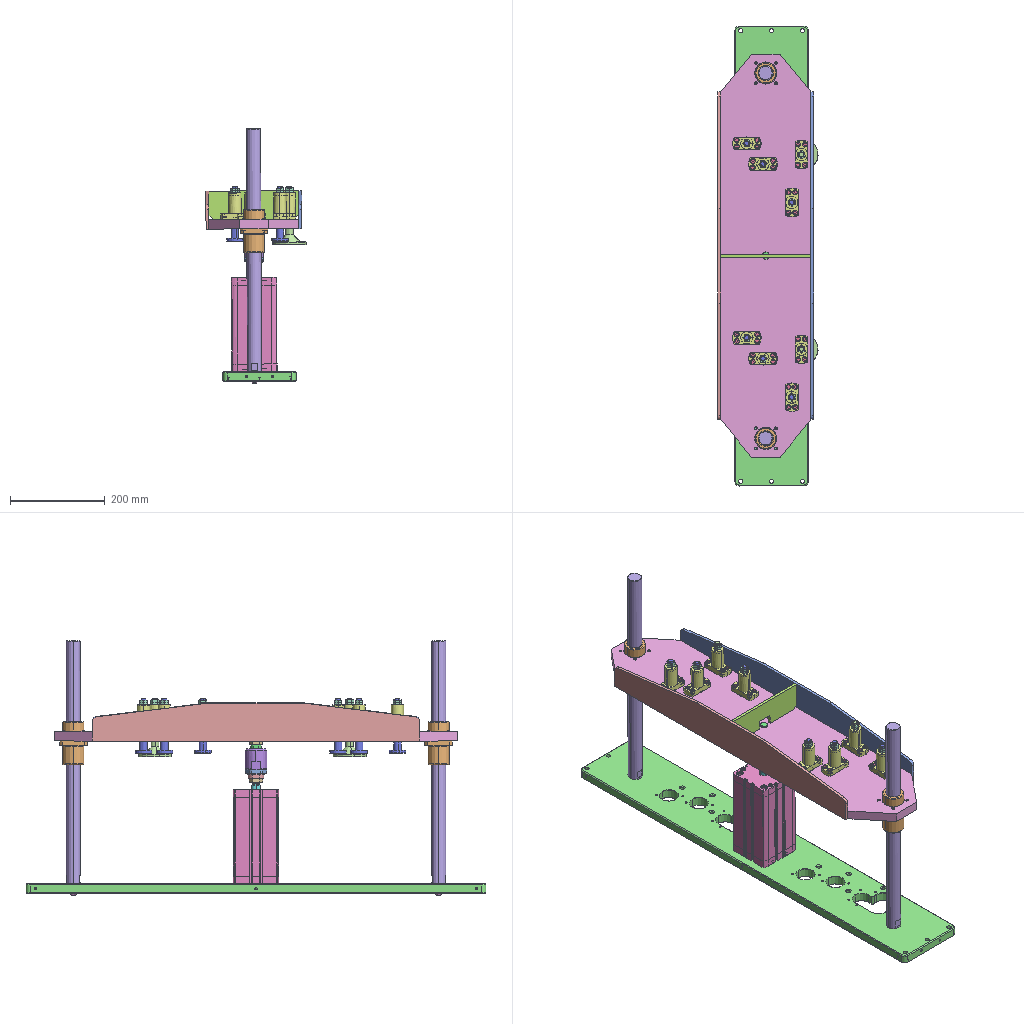Assembly | SolidWorks | 29 different items | 160 placed | box 211 x 970 x 537 mm
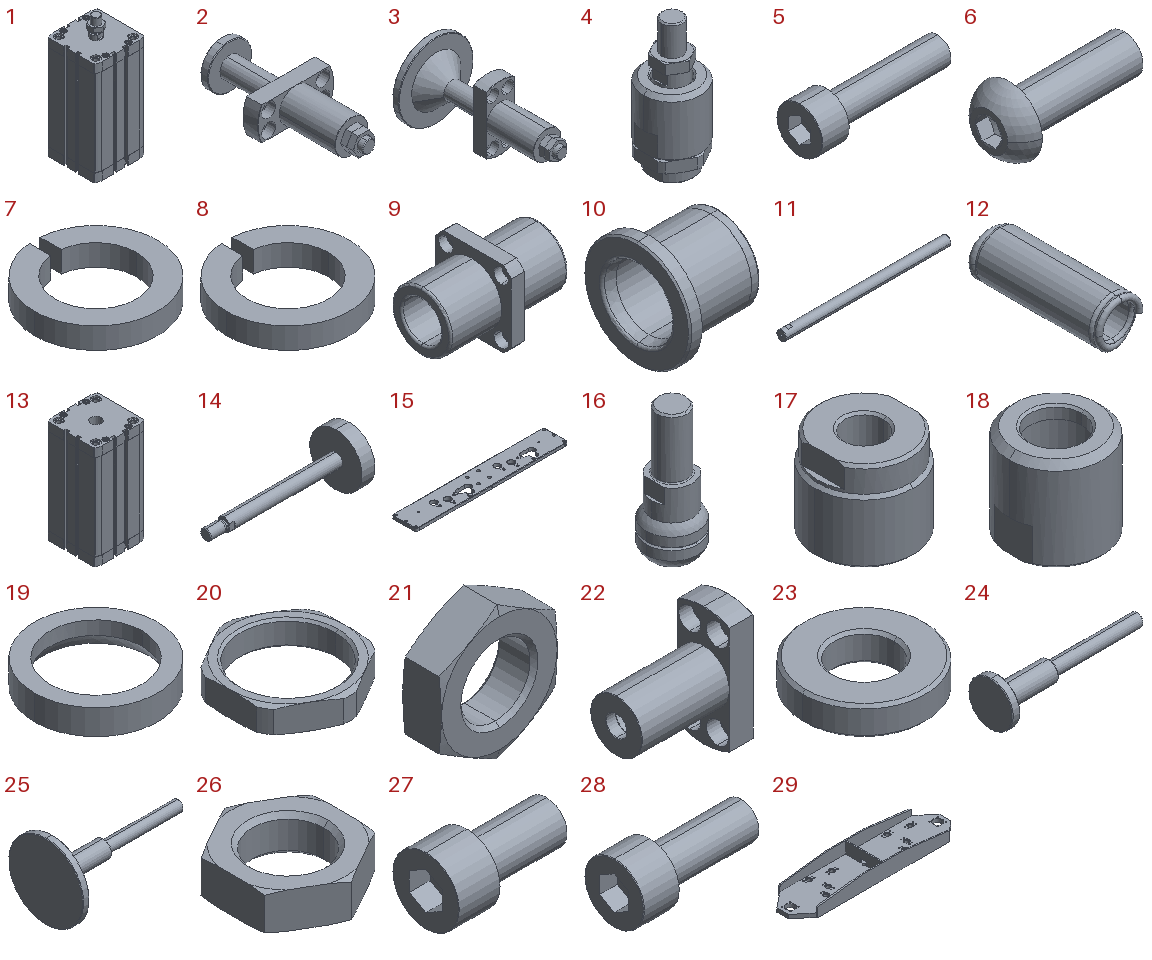Parts list (item | name | quantity | parent item | size | volume | features):
1 | (subassembly) | x1 | - | 95.5 x 95.5 x 235.9 mm | 1025771 mm3 | features AEMSimFeature 1
2 | (subassembly) | x6 | - | 60 x 116 x 35 mm | 44570 mm3 | features AEMSimFeature 1
3 | (subassembly) | x2 | - | 70 x 124 x 70 mm | 72658 mm3 | features AEMSimFeature 1
4 | (subassembly) | x1 | - | 45 x 45 x 103 mm | 90630 mm3 | features AEMSimFeature 1
5 | - | x8 | - | 31 x 10 x 10 mm | 1111 mm3 | features BlendCut 1, Cut 1, Fillet 1, LPattern 1, RevCut 1, Revolution 1
6 | - | x2 | - | 29.4 x 14 x 14 mm | 1672 mm3 | features RevCut 2, Revolution 2, Cut 1, LPattern 1, RefAxis 1
7 | - | x16 | - | 9.282 x 9.265 x 1.6 mm | 59.463 mm3 | features Extrusion 1
8 | - | x16 | - | 9.282 x 9.265 x 1.6 mm | 59.463 mm3 | features Extrusion 1
9 | - | x2 | - | 90 x 58 x 58 mm | 93231 mm3 | features ICE 3, CirPattern 1, Fillet 1, Revolution 1
10 | - | x8 | - | 20 x 26 x 26 mm | 2854 mm3 | features Revolution 1
11 | - | x2 | - | 525 x 30 x 30 mm | 369974 mm3 | features ICE 1, RevCut 1, Revolution 1
12 | - | x8 | in 2, 3 | 16 x 45 x 16 mm | 4068 mm3 | features Revolution 5, RevCut 1
13 | - | x1 | in 1 | 95.5 x 95.5 x 199 mm | 863513 mm3 | features BaseBody 1
14 | - | x1 | in 1 | 219.5 x 80 x 80 mm | 159613 mm3 | features BaseBody 1
15 | - | x1 | - | 970 x 155 x 20 mm | 2656838 mm3 | features Chamfer 10, 3DProfileFeature 8, HoleWzd 8, ICE 8, LPattern 6, Fillet 3, Extrusion 1
16 | - | x1 | in 4 | 27.8 x 27.8 x 69.5 mm | 24116 mm3 | features BaseBody 1
17 | - | x1 | in 4 | 36 x 36 x 32 mm | 25281 mm3 | features BaseBody 1
18 | - | x1 | in 4 | 45 x 45 x 44 mm | 29973 mm3 | features BaseBody 1
19 | - | x2 | in 4 | 32 x 32 x 6.5 mm | 2061 mm3 | features BaseBody 1
20 | - | x1 | in 4 | 41 x 45 x 9 mm | 4491 mm3 | features BaseBody 1
21 | - | x2 | in 1, 4 | 24 x 8 x 27.713 mm | 2646 mm3 | features BaseBody 1
22 | - | x8 | in 2, 3 | 56 x 26 x 60 mm | 18631 mm3 | features Chamfer 3, ICE 2, 3DProfileFeature 1, HoleWzd 1, Revolution 1
23 | - | x8 | in 2, 3 | 21.5 x 21.5 x 5 mm | 1357 mm3 | features Chamfer 1, Extrusion 1
24 | - | x6 | in 2 | 116 x 35 x 35 mm | 19276 mm3 | features Chamfer 2, Revolution 1
25 | - | x2 | in 3 | 124 x 70 x 70 mm | 47364 mm3 | features Chamfer 3, Revolution 1
26 | - | x16 | in 2, 3 | 15.424 x 17.77 x 5 mm | 619.089 mm3 | features Cut 2, Chamfer 1, Extrusion 1
27 | - | x4 | - | 30 x 16 x 16 mm | 3296 mm3 | features BlendCut 1, Cut 1, Fillet 1, LPattern 1, RevCut 1, Revolution 1
28 | - | x32 | - | 22 x 10 x 10 mm | 856.284 mm3 | features BlendCut 1, Cut 1, Fillet 1, LPattern 1, RevCut 1, Revolution 1
29 | - | x1 | - | 850.5 x 202 x 80 mm | 3525282 mm3 | features ICE 11, LPattern 6, 3DProfileFeature 4, HoleWzd 4, Chamfer 3, CirPattern 3, Extrusion 1, Fillet 1, MirrorPattern 1, MirrorSolid 1, WeldmentFeature 1
Mates (type | each side: item.copy, entity, surface, feature):
In the top assembly
Concentric | 29.1 face cylinder Cut-Extrude4 | 10.1 face cylinder Revolve1
Coincident | 29.1 face plane Cut-Extrude5 | 10.1 face plane Revolve1
Concentric | 29.1 face cylinder Cut-Extrude4 | 10.2 face cylinder Revolve1
Coincident | 29.1 face plane Cut-Extrude5 | 10.2 face plane Revolve1
Concentric | 29.1 face cylinder Cut-Extrude4 | 10.3 face cylinder Revolve1
Coincident | 29.1 face plane Cut-Extrude5 | 10.3 face plane Revolve1
Concentric | 29.1 face cylinder Cut-Extrude4 | 10.4 face cylinder Revolve1
Coincident | 29.1 face plane Cut-Extrude5 | 10.4 face plane Revolve1
Coincident | 29.1 face plane Boss-Extrude1 | 9.1 face plane Revolve1
Concentric | 9.1 face cylinder Revolve1 | 11.1 face cylinder Revolve1
Parallel | 29.1 face plane Boss-Extrude1 | 15.1 face plane Boss-Extrude1
Concentric | 11.1 face cylinder Revolve1 | 15.1 face cylinder Cut-Extrude4
Coincident | 11.1 face plane Revolve1 | 15.1 face plane Cut-Extrude4
Coincident | 28.1 face plane Base-Revolve | 7.1 face plane Extrude1
Concentric | 28.1 face cylinder Base-Revolve | 7.1 face cylinder Extrude1
Concentric | 15.1 face cylinder LPattern5 | 11.2 face cylinder Revolve1
Concentric | 29.1 face cylinder Mirror1 | 9.2 face cylinder Revolve1
Concentric | 11.2 face cylinder Revolve1 | 9.2 face cylinder Revolve1
Coincident | 29.1 face plane Boss-Extrude1 | 22.1 face plane Revolve1
Concentric | 10.5 face cylinder Revolve1 | 22.1 face cylinder Revolve1
Concentric | 29.1 face cylinder LPattern1 | 10.5 face cylinder Revolve1
Coincident | 29.1 face plane Boss-Extrude1 | 22.2 face plane Revolve1
Concentric | 10.6 face cylinder Revolve1 | 22.2 face cylinder Revolve1
Concentric | 29.1 face cylinder LPattern1 | 10.6 face cylinder Revolve1
Coincident | 29.1 face plane Boss-Extrude1 | 22.3 face plane Revolve1
Concentric | 10.7 face cylinder Revolve1 | 22.3 face cylinder Revolve1
Concentric | 29.1 face cylinder LPattern1 | 10.7 face cylinder Revolve1
Coincident | 29.1 face plane Boss-Extrude1 | 22.4 face plane Revolve1
Concentric | 10.8 face cylinder Revolve1 | 22.4 face cylinder Revolve1
Concentric | 29.1 face cylinder LPattern1 | 10.8 face cylinder Revolve1
Concentric | 14.1 face cylinder Input 1 | 18.1 face cylinder Input 1
Concentric | 29.1 face cylinder M16x1.5 Tapped Hole1 | 16.1 face cylinder Input 1
Parallel | 15.1 face plane Cut-Extrude7 | 13.1 face plane Input 1
Coincident | 15.1 face plane Boss-Extrude1 | 13.1 face plane Input 1
Concentric | 28.2 face cylinder Base-Revolve | 22.1 face cylinder Hole size per hex socket head cap screw type 1
Concentric | 7.2 face cylinder Extrude1 | 22.1 face cylinder Hole size per hex socket head cap screw type 1
Concentric | 29.1 face cylinder LPattern12 | 28.2 face cylinder Base-Revolve
Concentric | 28.3 face cylinder Base-Revolve | 22.2 face cylinder Hole size per hex socket head cap screw type 1
Concentric | 7.3 face cylinder Extrude1 | 28.3 face cylinder Base-Revolve
Concentric | 29.1 face cylinder LPattern12 | 28.3 face cylinder Base-Revolve
Concentric | 29.1 face cylinder LPattern12 | 22.3 face cylinder Hole size per hex socket head cap screw type 1
Concentric | 29.1 face cylinder LPattern6 | 22.4 face cylinder Hole size per hex socket head cap screw type 1
Concentric | 29.1 face cylinder LPattern13 | 9.2 face cylinder CirPattern1
Coincident | 15.1 face plane Boss-Extrude1 | 6.1 face plane Revolve1
Concentric | 11.2 face cylinder Cut-Revolve1 | 6.1 face cylinder Revolve1
Coincident | 9.2 face plane CirPattern1 | 5.1 face plane Base-Revolve
Concentric | 9.2 face cylinder CirPattern1 | 5.1 face cylinder Base-Revolve
Coincident | 28.4 face plane Base-Revolve | 8.1 face plane Extrude1
Concentric | 28.4 face cylinder Base-Revolve | 8.1 face cylinder Extrude1
Coincident | 22.3 face plane Hole size per hex socket head cap screw type 1 | 8.1 face plane Extrude1
Concentric | 22.3 face cylinder Hole size per hex socket head cap screw type 1 | 28.4 face cylinder Base-Revolve
Coincident | 15.1 face plane Hole size per hex socket head cap screw type 1 | 27.1 face plane Base-Revolve
Concentric | 15.1 face cylinder Hole size per hex socket head cap screw type 1 | 27.1 face cylinder Base-Revolve
In subassembly 2
Coincident | 22.5 axis | 12.1 axis
Coincident | 22.5 face plane Revolve1 | 23.1 face plane Boss-Extrude1
Concentric | 22.5 face cylinder Revolve1 | 23.1 face cylinder Boss-Extrude1
Concentric | 23.1 face cylinder Boss-Extrude1 | 24.1 face cylinder Revolve1
Coincident | 23.1 face plane Boss-Extrude1 | 24.1 face plane Revolve1
Lock | 23.1 select_type:0 | 12.1 select_type:0
Concentric | 26.1 face cylinder Base-Extrude | 26.2 face cylinder Base-Extrude
Coincident | 26.1 face plane Base-Extrude | 26.2 face plane Base-Extrude | 2 times
Coincident | 22.5 face plane Revolve1 | 26.2 face plane Base-Extrude
Concentric | 26.1 face cylinder Base-Extrude | 24.1 face cylinder Revolve1
Parallel | 22.5 face plane Cut-Extrude2 | 2.1 plane
In subassembly 3
Coincident | 22.5 axis | 12.1 axis
Coincident | 22.5 face plane Revolve1 | 23.1 face plane Boss-Extrude1
Concentric | 22.5 face cylinder Revolve1 | 23.1 face cylinder Boss-Extrude1
Concentric | 23.1 face cylinder Boss-Extrude1 | 25.1 face cylinder Revolve1
Coincident | 23.1 face plane Boss-Extrude1 | 25.1 face plane Revolve1
Lock | 23.1 select_type:0 | 12.1 select_type:0
Concentric | 26.1 face cylinder Base-Extrude | 26.2 face cylinder Base-Extrude
Coincident | 26.1 face plane Base-Extrude | 26.2 face plane Base-Extrude | 2 times
Coincident | 22.5 face plane Revolve1 | 26.2 face plane Base-Extrude
Concentric | 26.1 face cylinder Base-Extrude | 25.1 face cylinder Revolve1
Parallel | 22.5 face plane Cut-Extrude2 | 3.1 plane